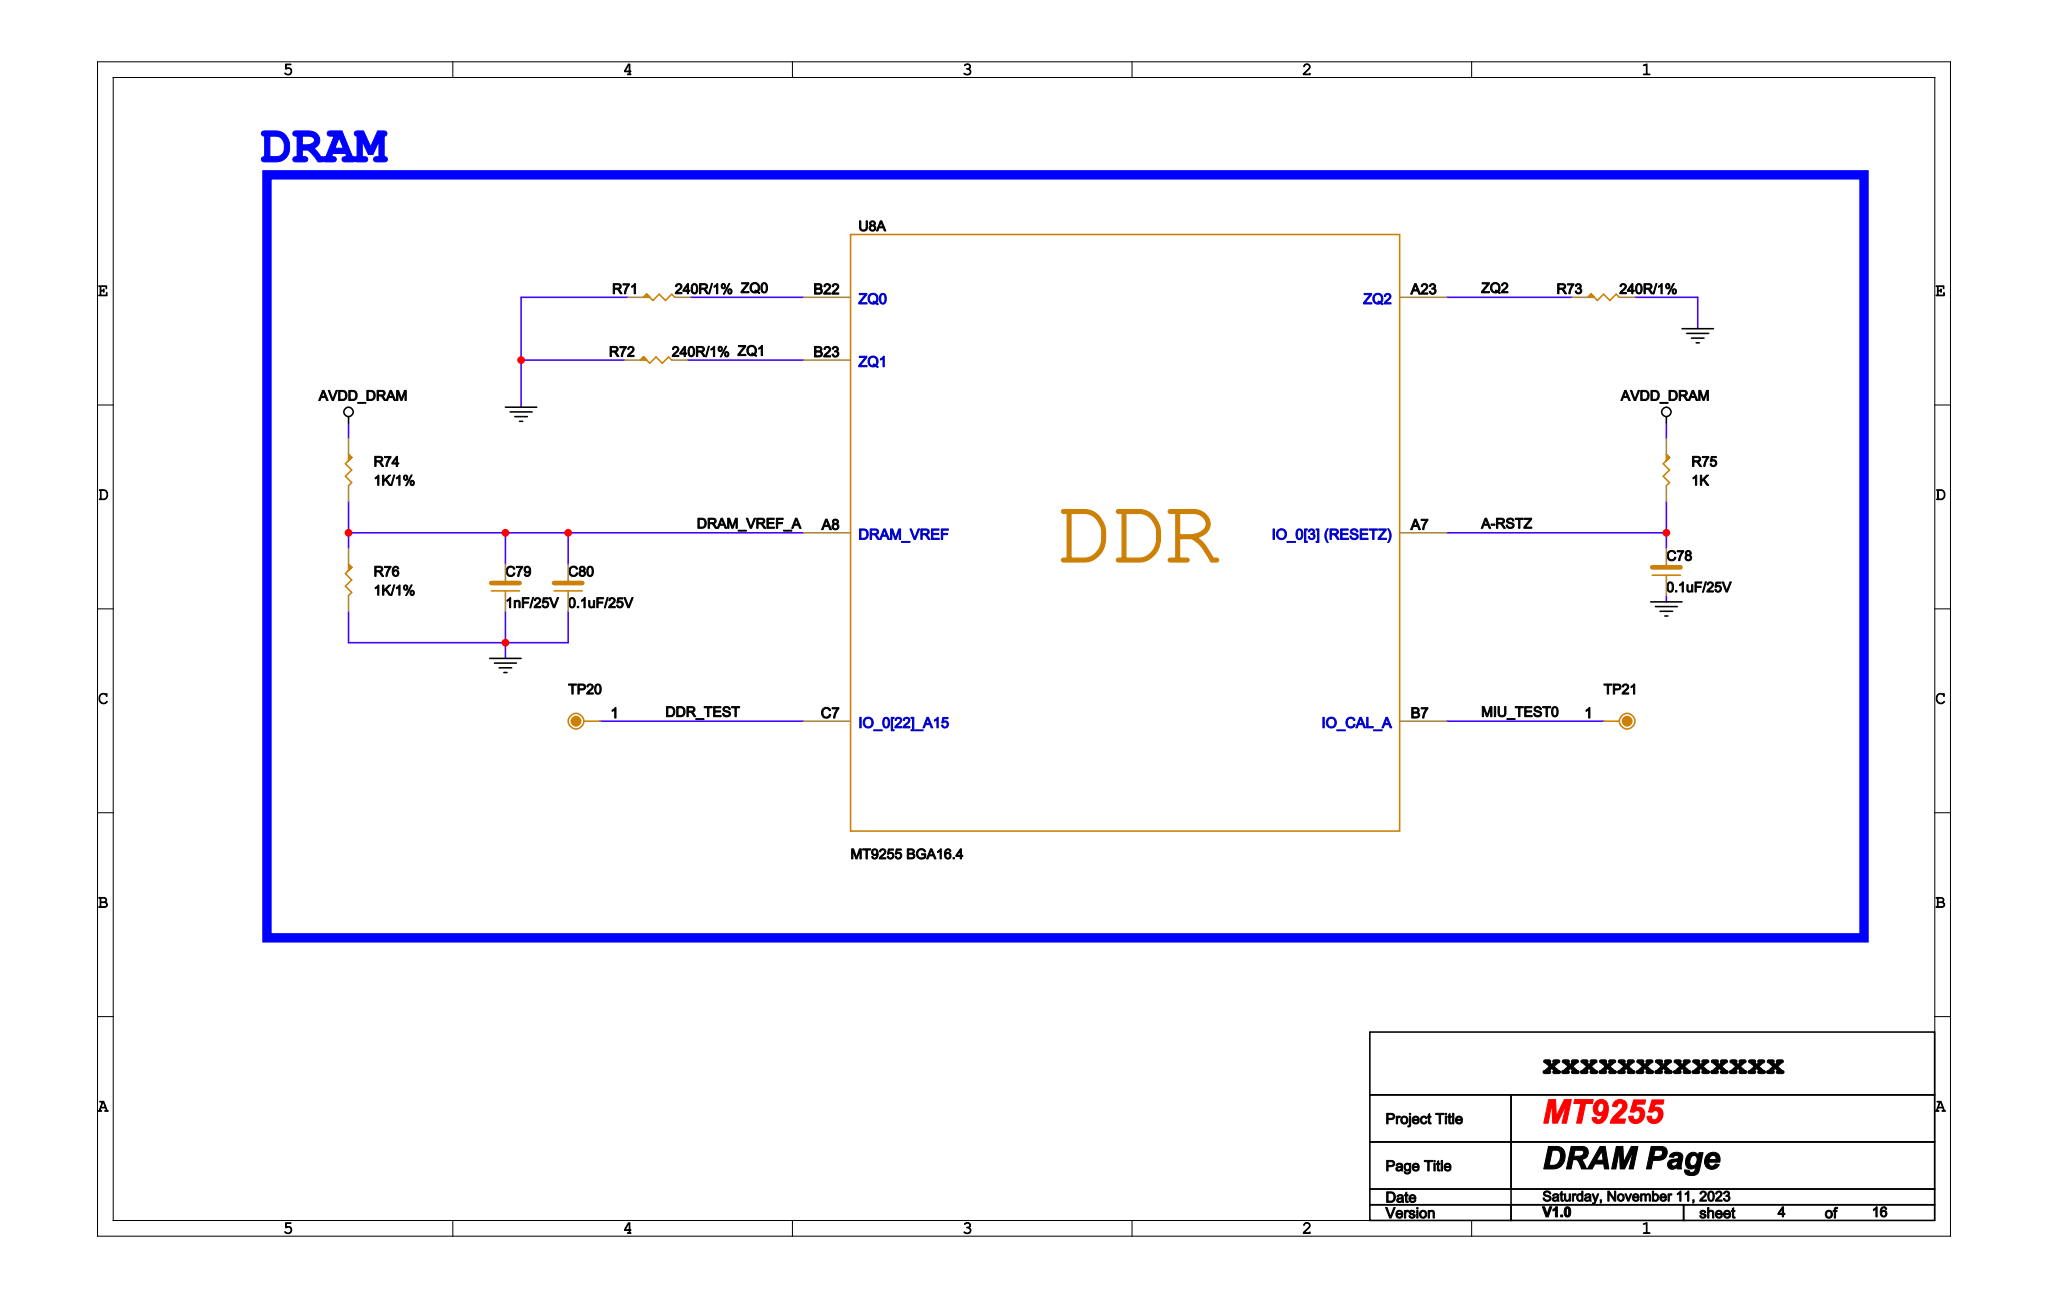Circuit board | Cadence Allegro | 1223 parts | 777 nets | one sheet of the schematic
Parts on this sheet (reference | value | footprint):
C78 | 0.1uF/25V | C0402
C79 | 1nF/25V | C0402
C80 | 0.1uF/25V | C0402
R71 | 240R/1% | R0402
R72 | 240R/1% | R0402
R73 | 240R/1% | R0402
R74 | 1K/1% | R0402
R75 | 1K | R0402
R76 | 1K/1% | R0402
TP20 | DEO | TP06MM
TP21 | DEO | TP06MM
U8 | MT9255 BGA16.4 | LFBGA462
Nets of these parts (net: part-pin ...):
GND: C78-2 C79-2 C80-2 R71-1 R72-1 R73-2 R76-2
+1.5V_DDR: R74-1 R75-1
A-RSTZ: C78-1 R75-2 U8-A7
DRAM_VREF_A: C79-1 C80-1 R74-2 R76-1 U8-A8
DDR_TEST: TP20-1 U8-C7
MIU_TEST0: TP21-1 U8-B7
ZQ0: R71-2 U8-B22
ZQ1: R72-2 U8-B23
ZQ2: R73-1 U8-A23